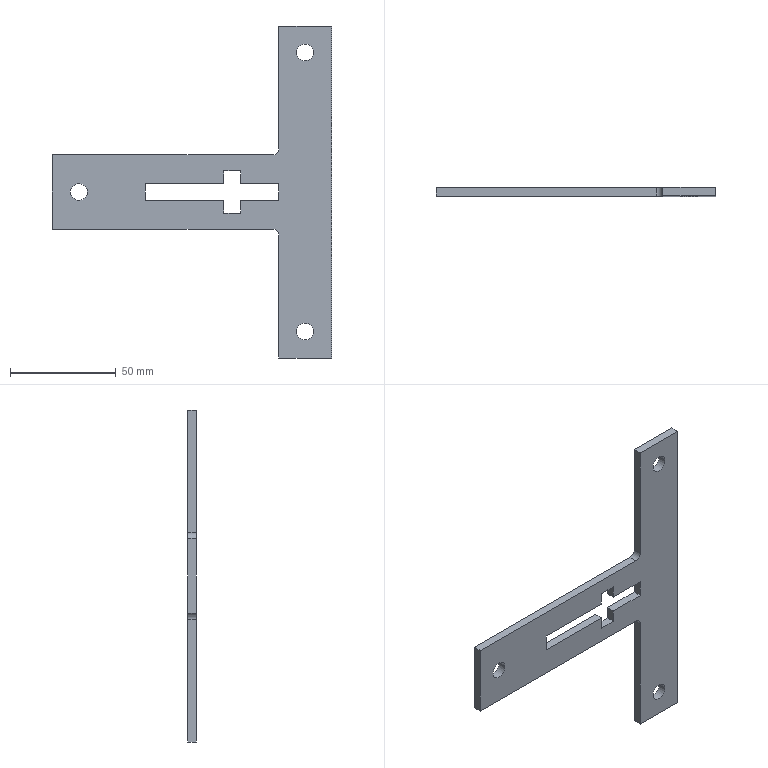Part | STEP file | 64562894 | 1 solid | 30 faces | box 132 x 4 x 157 mm | volume 27692 mm3 | plane 22 | cylinder 8 | commonest cylinder face diameters 8 x6 6 x2